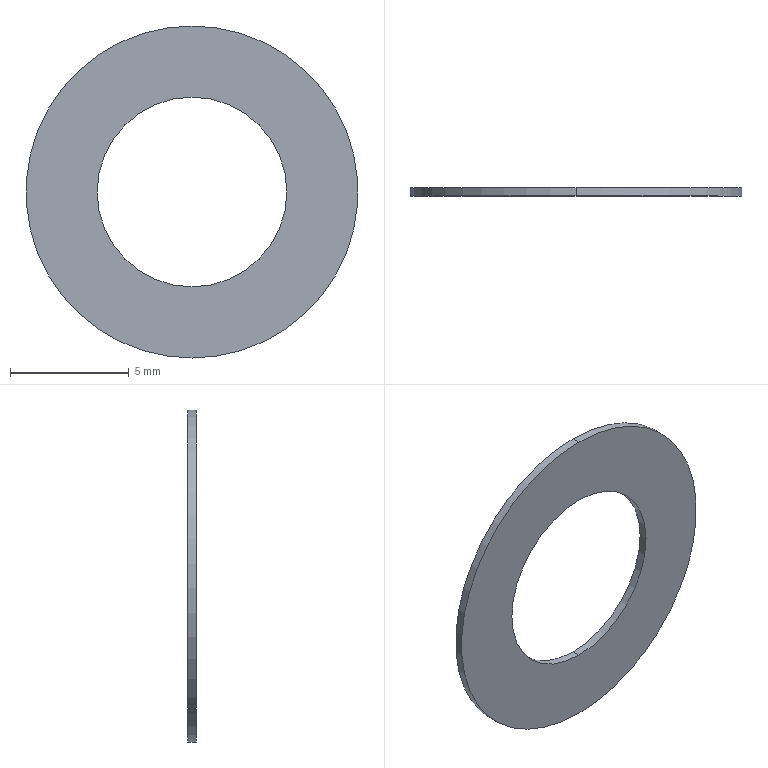Part | SolidWorks | features Extrusion 1 | 1 solid | 6 faces | box 14 x 0.35 x 14 mm | volume 36.285 mm3 | cylinder 4 | plane 2 | commonest cylinder face diameters 8 x2 14 x2
STEP:
#1=CARTESIAN_POINT('',(0.,0.35,-4.));
#2=VERTEX_POINT('',#1);
#3=CARTESIAN_POINT('',(0.,0.35,4.));
#4=VERTEX_POINT('',#3);
#5=CARTESIAN_POINT('',(0.,0.35,0.));
#6=DIRECTION('',(0.,1.,0.));
#7=DIRECTION('',(0.,0.,1.));
#8=AXIS2_PLACEMENT_3D('',#5,#6,#7);
#9=CIRCLE('',#8,4.);
#10=EDGE_CURVE('',#2,#4,#9,.T.);
#11=ORIENTED_EDGE('',*,*,#10,.T.);
#12=CARTESIAN_POINT('',(0.,0.,4.));
#13=VERTEX_POINT('',#12);
#14=CARTESIAN_POINT('',(0.,0.35,4.));
#15=DIRECTION('',(0.,-1.,0.));
#16=VECTOR('',#15,1000.);
#17=LINE('',#14,#16);
#18=EDGE_CURVE('',#4,#13,#17,.T.);
#19=ORIENTED_EDGE('',*,*,#18,.T.);
#20=CARTESIAN_POINT('',(0.,0.,-4.));
#21=VERTEX_POINT('',#20);
#22=CARTESIAN_POINT('',(0.,0.,0.));
#23=DIRECTION('',(0.,1.,0.));
#24=DIRECTION('',(0.,0.,1.));
#25=AXIS2_PLACEMENT_3D('',#22,#23,#24);
#26=CIRCLE('',#25,4.);
#27=EDGE_CURVE('',#21,#13,#26,.T.);
#28=ORIENTED_EDGE('',*,*,#27,.F.);
#29=CARTESIAN_POINT('',(0.,0.35,-4.));
#30=DIRECTION('',(0.,-1.,0.));
#31=VECTOR('',#30,1000.);
#32=LINE('',#29,#31);
#33=EDGE_CURVE('',#2,#21,#32,.T.);
#34=ORIENTED_EDGE('',*,*,#33,.F.);
#35=EDGE_LOOP('',(#11,#19,#28,#34));
#36=FACE_OUTER_BOUND('',#35,.T.);
#37=CARTESIAN_POINT('',(0.,0.35,0.));
#38=DIRECTION('',(0.,-1.,0.));
#39=DIRECTION('',(0.,0.,-1.));
#40=AXIS2_PLACEMENT_3D('',#37,#38,#39);
#41=CYLINDRICAL_SURFACE('',#40,4.);
#42=ADVANCED_FACE('',(#36),#41,.F.);
#43=CARTESIAN_POINT('',(0.,0.35,7.));
#44=VERTEX_POINT('',#43);
#45=CARTESIAN_POINT('',(0.,0.35,-7.));
#46=VERTEX_POINT('',#45);
#47=CARTESIAN_POINT('',(0.,0.35,0.));
#48=DIRECTION('',(0.,1.,0.));
#49=DIRECTION('',(0.,0.,1.));
#50=AXIS2_PLACEMENT_3D('',#47,#48,#49);
#51=CIRCLE('',#50,7.);
#52=EDGE_CURVE('',#44,#46,#51,.T.);
#53=ORIENTED_EDGE('',*,*,#52,.F.);
#54=CARTESIAN_POINT('',(0.,0.,7.));
#55=VERTEX_POINT('',#54);
#56=CARTESIAN_POINT('',(0.,0.35,7.));
#57=DIRECTION('',(0.,-1.,0.));
#58=VECTOR('',#57,1000.);
#59=LINE('',#56,#58);
#60=EDGE_CURVE('',#44,#55,#59,.T.);
#61=ORIENTED_EDGE('',*,*,#60,.T.);
#62=CARTESIAN_POINT('',(0.,0.,-7.));
#63=VERTEX_POINT('',#62);
#64=CARTESIAN_POINT('',(0.,0.,0.));
#65=DIRECTION('',(0.,1.,0.));
#66=DIRECTION('',(0.,0.,1.));
#67=AXIS2_PLACEMENT_3D('',#64,#65,#66);
#68=CIRCLE('',#67,7.);
#69=EDGE_CURVE('',#55,#63,#68,.T.);
#70=ORIENTED_EDGE('',*,*,#69,.T.);
#71=CARTESIAN_POINT('',(0.,0.35,-7.));
#72=DIRECTION('',(0.,-1.,0.));
#73=VECTOR('',#72,1000.);
#74=LINE('',#71,#73);
#75=EDGE_CURVE('',#46,#63,#74,.T.);
#76=ORIENTED_EDGE('',*,*,#75,.F.);
#77=EDGE_LOOP('',(#53,#61,#70,#76));
#78=FACE_OUTER_BOUND('',#77,.T.);
#79=CARTESIAN_POINT('',(0.,0.35,0.));
#80=DIRECTION('',(0.,-1.,0.));
#81=DIRECTION('',(0.,0.,-1.));
#82=AXIS2_PLACEMENT_3D('',#79,#80,#81);
#83=CYLINDRICAL_SURFACE('',#82,7.);
#84=ADVANCED_FACE('',(#78),#83,.T.);
#85=CARTESIAN_POINT('',(0.,0.35,0.));
#86=DIRECTION('',(0.,1.,0.));
#87=DIRECTION('',(0.,0.,1.));
#88=AXIS2_PLACEMENT_3D('',#85,#86,#87);
#89=CIRCLE('',#88,7.);
#90=EDGE_CURVE('',#46,#44,#89,.T.);
#91=ORIENTED_EDGE('',*,*,#90,.T.);
#92=ORIENTED_EDGE('',*,*,#52,.T.);
#93=EDGE_LOOP('',(#91,#92));
#94=FACE_OUTER_BOUND('',#93,.T.);
#95=ORIENTED_EDGE('',*,*,#10,.F.);
#96=CARTESIAN_POINT('',(0.,0.35,0.));
#97=DIRECTION('',(0.,1.,0.));
#98=DIRECTION('',(0.,0.,1.));
#99=AXIS2_PLACEMENT_3D('',#96,#97,#98);
#100=CIRCLE('',#99,4.);
#101=EDGE_CURVE('',#4,#2,#100,.T.);
#102=ORIENTED_EDGE('',*,*,#101,.F.);
#103=EDGE_LOOP('',(#95,#102));
#104=FACE_BOUND('',#103,.T.);
#105=CARTESIAN_POINT('',(0.,0.35,0.));
#106=DIRECTION('',(0.,1.,0.));
#107=DIRECTION('',(0.,0.,1.));
#108=AXIS2_PLACEMENT_3D('',#105,#106,#107);
#109=PLANE('',#108);
#110=ADVANCED_FACE('',(#94,#104),#109,.T.);
#111=CARTESIAN_POINT('',(0.,0.,0.));
#112=DIRECTION('',(0.,1.,0.));
#113=DIRECTION('',(0.,0.,1.));
#114=AXIS2_PLACEMENT_3D('',#111,#112,#113);
#115=CIRCLE('',#114,7.);
#116=EDGE_CURVE('',#63,#55,#115,.T.);
#117=ORIENTED_EDGE('',*,*,#116,.F.);
#118=ORIENTED_EDGE('',*,*,#69,.F.);
#119=EDGE_LOOP('',(#117,#118));
#120=FACE_OUTER_BOUND('',#119,.T.);
#121=ORIENTED_EDGE('',*,*,#27,.T.);
#122=CARTESIAN_POINT('',(0.,0.,0.));
#123=DIRECTION('',(0.,1.,0.));
#124=DIRECTION('',(0.,0.,1.));
#125=AXIS2_PLACEMENT_3D('',#122,#123,#124);
#126=CIRCLE('',#125,4.);
#127=EDGE_CURVE('',#13,#21,#126,.T.);
#128=ORIENTED_EDGE('',*,*,#127,.T.);
#129=EDGE_LOOP('',(#121,#128));
#130=FACE_BOUND('',#129,.T.);
#131=CARTESIAN_POINT('',(0.,0.,0.));
#132=DIRECTION('',(0.,1.,0.));
#133=DIRECTION('',(0.,0.,1.));
#134=AXIS2_PLACEMENT_3D('',#131,#132,#133);
#135=PLANE('',#134);
#136=ADVANCED_FACE('',(#120,#130),#135,.F.);
#137=ORIENTED_EDGE('',*,*,#60,.F.);
#138=ORIENTED_EDGE('',*,*,#90,.F.);
#139=ORIENTED_EDGE('',*,*,#75,.T.);
#140=ORIENTED_EDGE('',*,*,#116,.T.);
#141=EDGE_LOOP('',(#137,#138,#139,#140));
#142=FACE_OUTER_BOUND('',#141,.T.);
#143=CARTESIAN_POINT('',(0.,0.35,0.));
#144=DIRECTION('',(0.,-1.,0.));
#145=DIRECTION('',(0.,0.,-1.));
#146=AXIS2_PLACEMENT_3D('',#143,#144,#145);
#147=CYLINDRICAL_SURFACE('',#146,7.);
#148=ADVANCED_FACE('',(#142),#147,.T.);
#149=ORIENTED_EDGE('',*,*,#18,.F.);
#150=ORIENTED_EDGE('',*,*,#101,.T.);
#151=ORIENTED_EDGE('',*,*,#33,.T.);
#152=ORIENTED_EDGE('',*,*,#127,.F.);
#153=EDGE_LOOP('',(#149,#150,#151,#152));
#154=FACE_OUTER_BOUND('',#153,.T.);
#155=CARTESIAN_POINT('',(0.,0.35,0.));
#156=DIRECTION('',(0.,-1.,0.));
#157=DIRECTION('',(0.,0.,-1.));
#158=AXIS2_PLACEMENT_3D('',#155,#156,#157);
#159=CYLINDRICAL_SURFACE('',#158,4.);
#160=ADVANCED_FACE('',(#154),#159,.F.);
#161=CLOSED_SHELL('',(#42,#84,#110,#136,#148,#160));
#162=MANIFOLD_SOLID_BREP('',#161);
#163=CARTESIAN_POINT('',(0.,0.,0.));
#164=DIRECTION('',(0.,0.,1.));
#165=DIRECTION('',(1.,0.,0.));
#166=AXIS2_PLACEMENT_3D('',#163,#164,#165);
#167=(LENGTH_UNIT()NAMED_UNIT(*)SI_UNIT(.MILLI.,.METRE.));
#168=UNCERTAINTY_MEASURE_WITH_UNIT(LENGTH_MEASURE(0.00001),#167,'','');
#169=(NAMED_UNIT(*)PLANE_ANGLE_UNIT()SI_UNIT($,.RADIAN.));
#170=(NAMED_UNIT(*)SI_UNIT($,.STERADIAN.)SOLID_ANGLE_UNIT());
#171=(GEOMETRIC_REPRESENTATION_CONTEXT(3)GLOBAL_UNCERTAINTY_ASSIGNED_CONTEXT((#168))GLOBAL_UNIT_ASSIGNED_CONTEXT((#167,#169,#170))REPRESENTATION_CONTEXT('',''));
#172=ADVANCED_BREP_SHAPE_REPRESENTATION('',(#162,#166),#171);